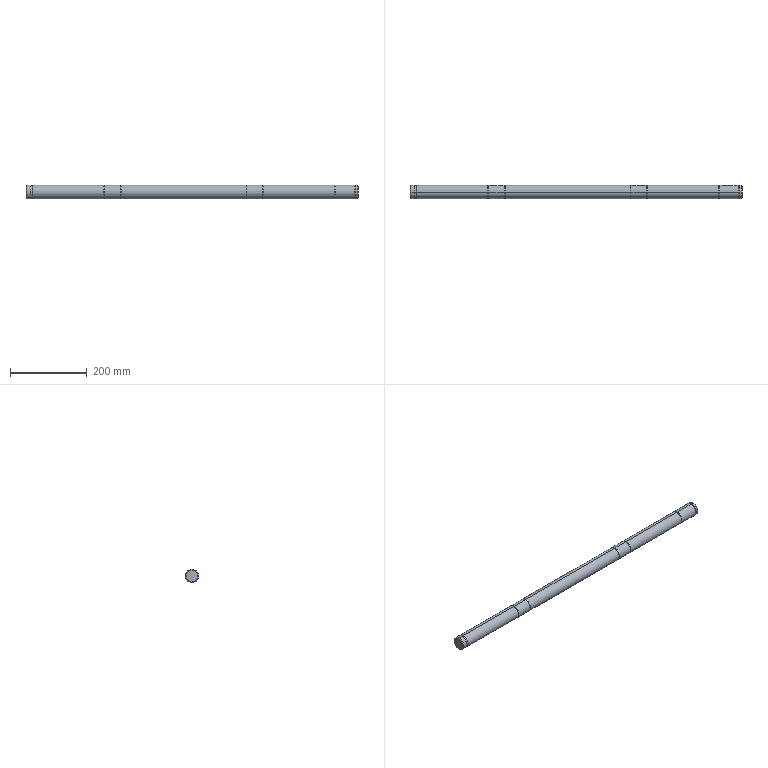Part | STEP file | IN-01-20-01_1 | 1 solid | 63 faces | box 865 x 35 x 35 mm | volume 826460 mm3 | cylinder 34 | plane 23 | cone 4 | spline 2 | commonest cylinder face diameters 35 x16 33 x12 10 x6